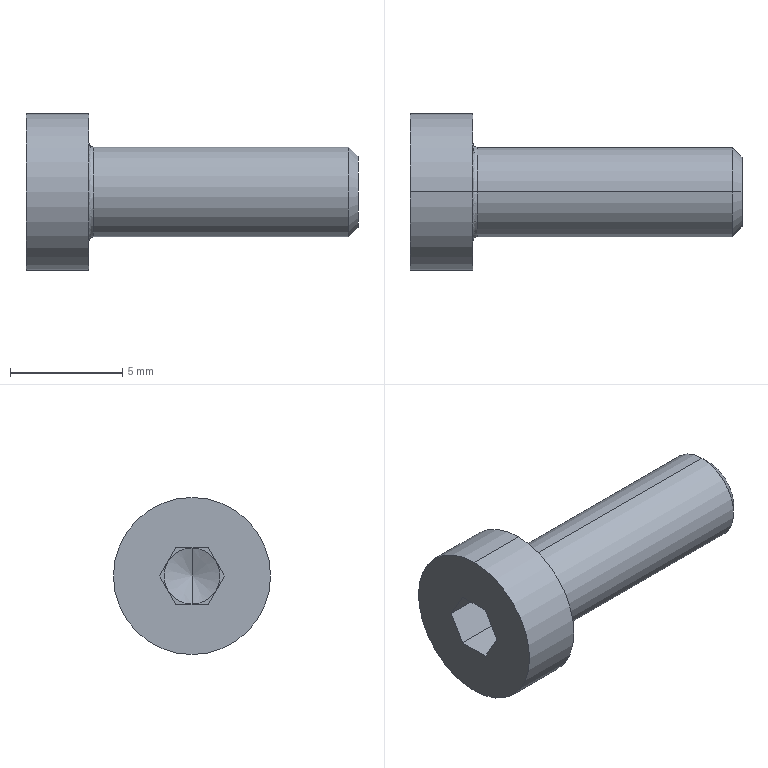Part | STEP file | SHTNZ12-25_2 | 1 solid | 25 faces | box 14.8 x 7 x 7 mm | volume 244.398 mm3 | plane 15 | cylinder 4 | cone 4 | spline 2 | commonest cylinder face diameters 4 x2 7 x2